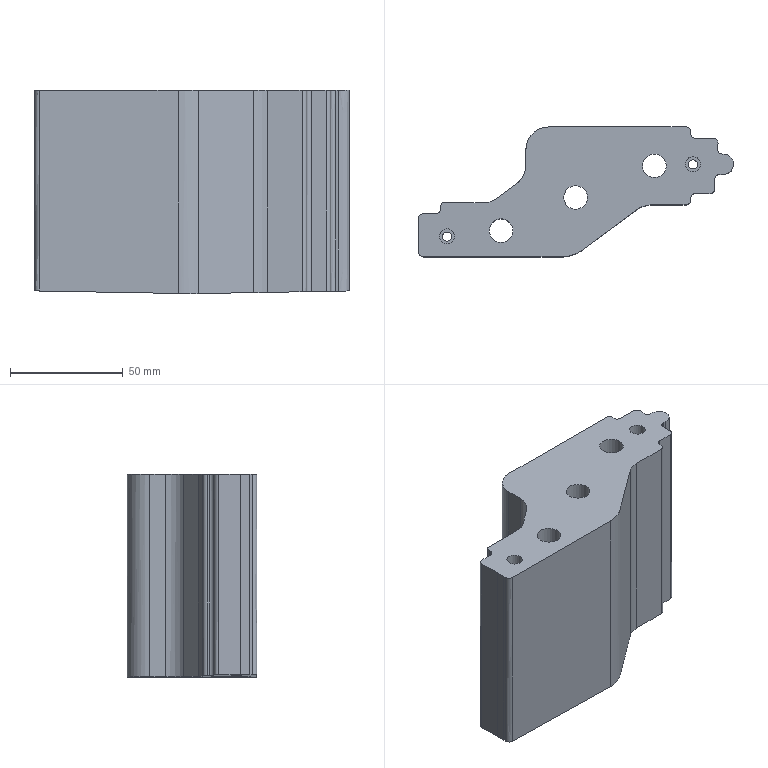Part | STEP file | gslz 2016.10.28-10_id2798_x_t | 1 solid | 60 faces | box 139.573 x 57.5 x 90 mm | volume 377716 mm3 | plane 24 | cylinder 24 | other 10 | spline 2 | commonest cylinder face diameters 4 x9 20 x4 10.5 x3 17 x3 4.1 x2 6.8 x2